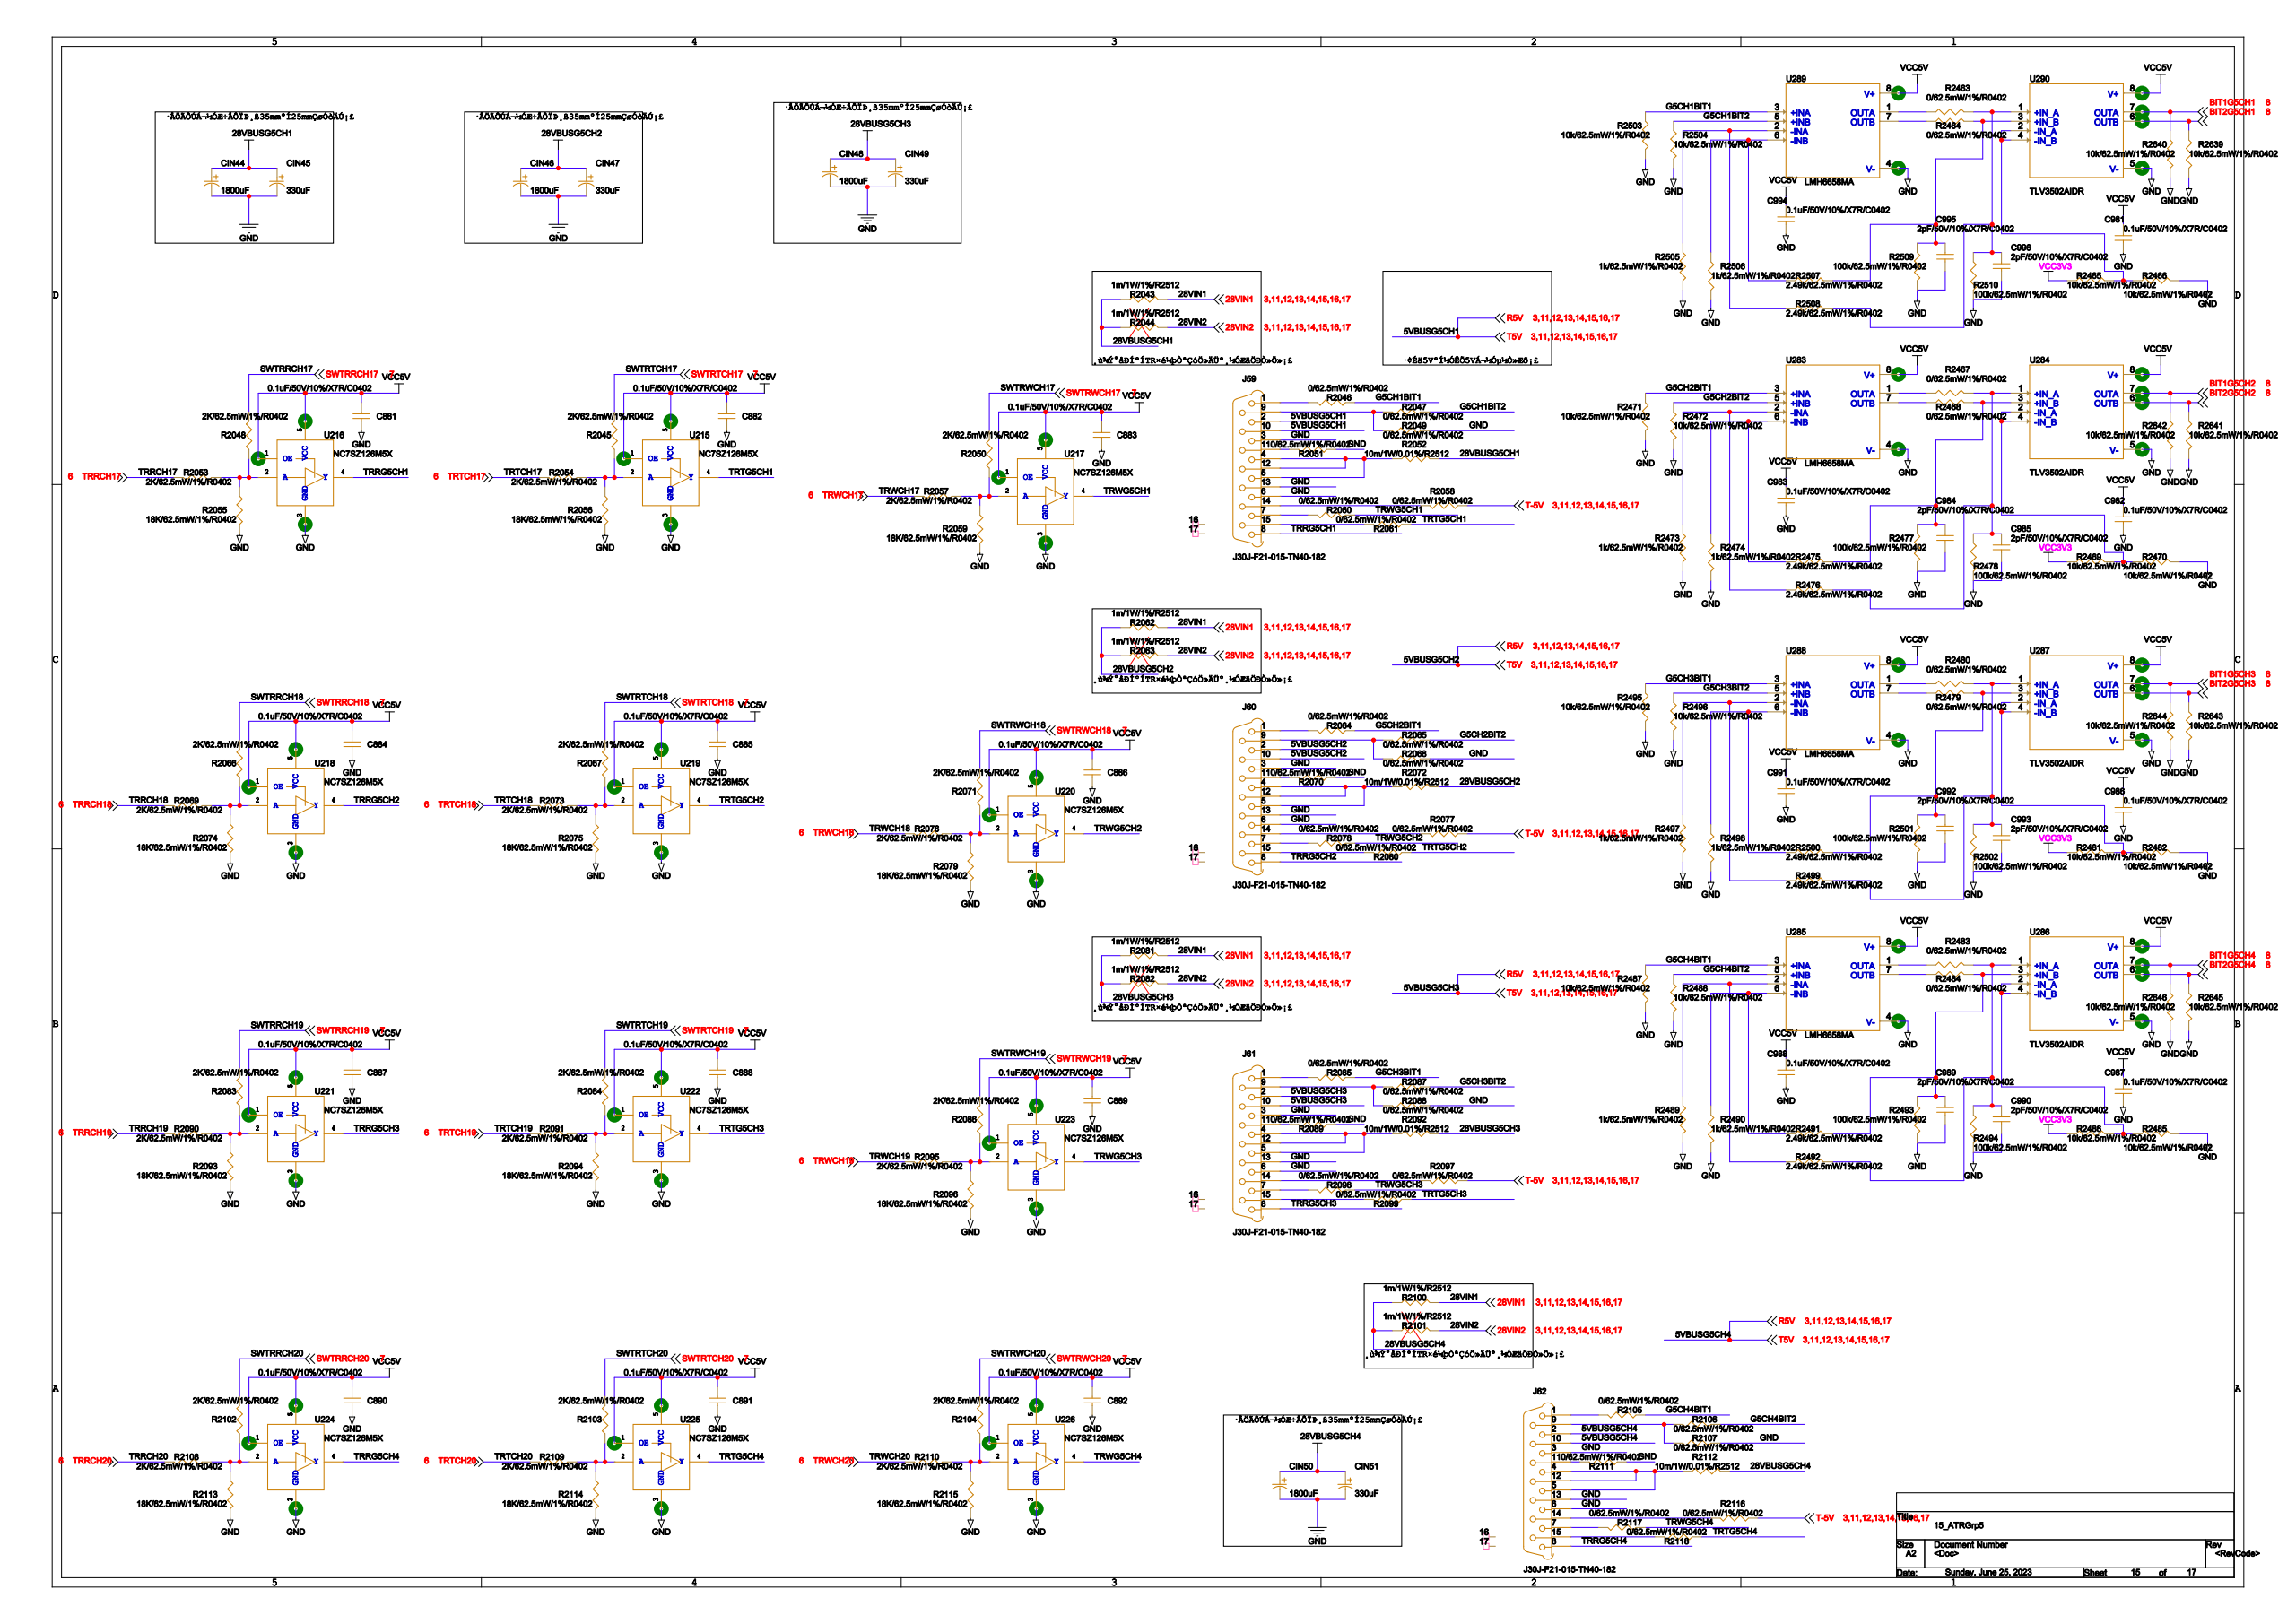Circuit board | Cadence Allegro | 1997 parts | 1536 nets | one sheet of the schematic
Parts on this sheet (reference | value | footprint):
C881 | 0.1uF/50V/10%/X7R/C0402 | 0402
C882 | 0.1uF/50V/10%/X7R/C0402 | 0402
C883 | 0.1uF/50V/10%/X7R/C0402 | 0402
C884 | 0.1uF/50V/10%/X7R/C0402 | 0402
C885 | 0.1uF/50V/10%/X7R/C0402 | 0402
C886 | 0.1uF/50V/10%/X7R/C0402 | 0402
C887 | 0.1uF/50V/10%/X7R/C0402 | 0402
C888 | 0.1uF/50V/10%/X7R/C0402 | 0402
C889 | 0.1uF/50V/10%/X7R/C0402 | 0402
C890 | 0.1uF/50V/10%/X7R/C0402 | 0402
C891 | 0.1uF/50V/10%/X7R/C0402 | 0402
C892 | 0.1uF/50V/10%/X7R/C0402 | 0402
C981 | 0.1uF/50V/10%/X7R/C0402 | 0402
C982 | 0.1uF/50V/10%/X7R/C0402 | 0402
C984 | 2pF/50V/10%/X7R/C0402 | 0402
C985 | 2pF/50V/10%/X7R/C0402 | 0402
C986 | 0.1uF/50V/10%/X7R/C0402 | 0402
C987 | 0.1uF/50V/10%/X7R/C0402 | 0402
C989 | 2pF/50V/10%/X7R/C0402 | 0402
C990 | 2pF/50V/10%/X7R/C0402 | 0402
C992 | 2pF/50V/10%/X7R/C0402 | 0402
C993 | 2pF/50V/10%/X7R/C0402 | 0402
C995 | 2pF/50V/10%/X7R/C0402 | 0402
C996 | 2pF/50V/10%/X7R/C0402 | 0402
CIN44 | ECF1HM182M27OTPO | AP-SMD_BD18-L27-W6_6-LS7_21
CIN45 | ECF1JM331G20OTPO | AP-SMD_BD10-L20-W6_6-LS7_21
CIN46 | ECF1HM182M27OTPO | AP-SMD_BD18-L27-W6_6-LS7_21
CIN47 | ECF1JM331G20OTPO | AP-SMD_BD10-L20-W6_6-LS7_21
CIN48 | ECF1HM182M27OTPO | AP-SMD_BD18-L27-W6_6-LS7_21
CIN49 | ECF1JM331G20OTPO | AP-SMD_BD10-L20-W6_6-LS7_21
CIN50 | ECF1HM182M27OTPO | AP-SMD_BD18-L27-W6_6-LS7_21
CIN51 | ECF1JM331G20OTPO | AP-SMD_BD10-L20-W6_6-LS7_21
J59 | J30J-F21-015-TN40-182 | J30J-F21-015-TN40-182
J60 | J30J-F21-015-TN40-182 | J30J-F21-015-TN40-182
J61 | J30J-F21-015-TN40-182 | J30J-F21-015-TN40-182
J62 | J30J-F21-015-TN40-182 | J30J-F21-015-TN40-182
R2043 | 1m/1W/1%/R2512 | 2512
R2044 | 1m/1W/1%/R2512 | 2512
R2045 | 2K/62.5mW/1%/R0402 | 0402
R2046 | 0/62.5mW/1%/R0402 | 0402
R2047 | 0/62.5mW/1%/R0402 | 0402
R2048 | 2K/62.5mW/1%/R0402 | 0402
R2049 | 0/62.5mW/1%/R0402 | 0402
R2050 | 2K/62.5mW/1%/R0402 | 0402
R2051 | 0/62.5mW/1%/R0402 | 0402
R2052 | 10m/1W/0.01%/R2512 | 2512
R2053 | 2K/62.5mW/1%/R0402 | 0402
R2054 | 2K/62.5mW/1%/R0402 | 0402
R2055 | 18K/62.5mW/1%/R0402 | 0402
R2056 | 18K/62.5mW/1%/R0402 | 0402
R2057 | 2K/62.5mW/1%/R0402 | 0402
R2058 | 0/62.5mW/1%/R0402 | 0402
R2059 | 18K/62.5mW/1%/R0402 | 0402
R2060 | 0/62.5mW/1%/R0402 | 0402
R2061 | 0/62.5mW/1%/R0402 | 0402
R2062 | 1m/1W/1%/R2512 | 2512
R2063 | 1m/1W/1%/R2512 | 2512
R2064 | 0/62.5mW/1%/R0402 | 0402
R2065 | 0/62.5mW/1%/R0402 | 0402
R2066 | 2K/62.5mW/1%/R0402 | 0402
R2067 | 2K/62.5mW/1%/R0402 | 0402
R2068 | 0/62.5mW/1%/R0402 | 0402
R2069 | 2K/62.5mW/1%/R0402 | 0402
R2070 | 0/62.5mW/1%/R0402 | 0402
R2071 | 2K/62.5mW/1%/R0402 | 0402
R2072 | 10m/1W/0.01%/R2512 | 2512
R2073 | 2K/62.5mW/1%/R0402 | 0402
R2074 | 18K/62.5mW/1%/R0402 | 0402
R2075 | 18K/62.5mW/1%/R0402 | 0402
R2076 | 2K/62.5mW/1%/R0402 | 0402
R2077 | 0/62.5mW/1%/R0402 | 0402
R2078 | 0/62.5mW/1%/R0402 | 0402
R2079 | 18K/62.5mW/1%/R0402 | 0402
R2080 | 0/62.5mW/1%/R0402 | 0402
R2081 | 1m/1W/1%/R2512 | 2512
R2082 | 1m/1W/1%/R2512 | 2512
R2083 | 2K/62.5mW/1%/R0402 | 0402
R2084 | 2K/62.5mW/1%/R0402 | 0402
R2085 | 0/62.5mW/1%/R0402 | 0402
R2086 | 2K/62.5mW/1%/R0402 | 0402
R2087 | 0/62.5mW/1%/R0402 | 0402
R2088 | 0/62.5mW/1%/R0402 | 0402
R2089 | 0/62.5mW/1%/R0402 | 0402
R2090 | 2K/62.5mW/1%/R0402 | 0402
R2091 | 2K/62.5mW/1%/R0402 | 0402
R2092 | 10m/1W/0.01%/R2512 | 2512
R2093 | 18K/62.5mW/1%/R0402 | 0402
R2094 | 18K/62.5mW/1%/R0402 | 0402
R2095 | 2K/62.5mW/1%/R0402 | 0402
R2096 | 18K/62.5mW/1%/R0402 | 0402
R2097 | 0/62.5mW/1%/R0402 | 0402
R2098 | 0/62.5mW/1%/R0402 | 0402
R2099 | 0/62.5mW/1%/R0402 | 0402
R2100 | 1m/1W/1%/R2512 | 2512
R2101 | 1m/1W/1%/R2512 | 2512
R2102 | 2K/62.5mW/1%/R0402 | 0402
R2103 | 2K/62.5mW/1%/R0402 | 0402
R2104 | 2K/62.5mW/1%/R0402 | 0402
R2105 | 0/62.5mW/1%/R0402 | 0402
R2106 | 0/62.5mW/1%/R0402 | 0402
R2107 | 0/62.5mW/1%/R0402 | 0402
R2108 | 2K/62.5mW/1%/R0402 | 0402
R2109 | 2K/62.5mW/1%/R0402 | 0402
R2110 | 2K/62.5mW/1%/R0402 | 0402
R2111 | 0/62.5mW/1%/R0402 | 0402
R2112 | 10m/1W/0.01%/R2512 | 2512
R2113 | 18K/62.5mW/1%/R0402 | 0402
R2114 | 18K/62.5mW/1%/R0402 | 0402
R2115 | 18K/62.5mW/1%/R0402 | 0402
R2116 | 0/62.5mW/1%/R0402 | 0402
R2117 | 0/62.5mW/1%/R0402 | 0402
R2118 | 0/62.5mW/1%/R0402 | 0402
R2463 | 0/62.5mW/1%/R0402 | 0402
R2464 | 0/62.5mW/1%/R0402 | 0402
R2465 | 10k/62.5mW/1%/R0402 | 0402
R2466 | 10k/62.5mW/1%/R0402 | 0402
R2467 | 0/62.5mW/1%/R0402 | 0402
R2468 | 0/62.5mW/1%/R0402 | 0402
R2469 | 10k/62.5mW/1%/R0402 | 0402
R2470 | 10k/62.5mW/1%/R0402 | 0402
R2471 | 10k/62.5mW/1%/R0402 | 0402
R2472 | 10k/62.5mW/1%/R0402 | 0402
R2473 | 1K/62.5mW/1%/R0402 | 0402
R2474 | 1K/62.5mW/1%/R0402 | 0402
R2476 | 2.49k/62.5mW/1%/R0402 | 0402
R2477 | 100k/62.5mW/1%/R0402 | 0402
R2478 | 100k/62.5mW/1%/R0402 | 0402
R2479 | 0/62.5mW/1%/R0402 | 0402
R2480 | 0/62.5mW/1%/R0402 | 0402
R2481 | 10k/62.5mW/1%/R0402 | 0402
R2482 | 10k/62.5mW/1%/R0402 | 0402
R2483 | 0/62.5mW/1%/R0402 | 0402
R2484 | 0/62.5mW/1%/R0402 | 0402
R2485 | 10k/62.5mW/1%/R0402 | 0402
R2486 | 10k/62.5mW/1%/R0402 | 0402
R2487 | 10k/62.5mW/1%/R0402 | 0402
R2488 | 10k/62.5mW/1%/R0402 | 0402
R2489 | 1K/62.5mW/1%/R0402 | 0402
R2490 | 1K/62.5mW/1%/R0402 | 0402
R2492 | 2.49k/62.5mW/1%/R0402 | 0402
R2493 | 100k/62.5mW/1%/R0402 | 0402
R2494 | 100k/62.5mW/1%/R0402 | 0402
R2495 | 10k/62.5mW/1%/R0402 | 0402
R2496 | 10k/62.5mW/1%/R0402 | 0402
R2497 | 1K/62.5mW/1%/R0402 | 0402
R2498 | 1K/62.5mW/1%/R0402 | 0402
R2499 | 2.49k/62.5mW/1%/R0402 | 0402
R2500 | 2.49k/62.5mW/1%/R0402 | 0402
R2501 | 100k/62.5mW/1%/R0402 | 0402
R2502 | 100k/62.5mW/1%/R0402 | 0402
R2503 | 10k/62.5mW/1%/R0402 | 0402
R2504 | 10k/62.5mW/1%/R0402 | 0402
R2505 | 1K/62.5mW/1%/R0402 | 0402
R2506 | 1K/62.5mW/1%/R0402 | 0402
R2508 | 2.49k/62.5mW/1%/R0402 | 0402
R2509 | 100k/62.5mW/1%/R0402 | 0402
R2510 | 100k/62.5mW/1%/R0402 | 0402
R2639 | 10k/62.5mW/1%/R0402 | 0402
R2640 | 10k/62.5mW/1%/R0402 | 0402
R2641 | 10k/62.5mW/1%/R0402 | 0402
R2642 | 10k/62.5mW/1%/R0402 | 0402
R2643 | 10k/62.5mW/1%/R0402 | 0402
R2644 | 10k/62.5mW/1%/R0402 | 0402
R2645 | 10k/62.5mW/1%/R0402 | 0402
R2646 | 10k/62.5mW/1%/R0402 | 0402
U215 | NC7SZ126M5X | SOT-23-5
U216 | NC7SZ126M5X | SOT-23-5
U217 | NC7SZ126M5X | SOT-23-5
U218 | NC7SZ126M5X | SOT-23-5
U219 | NC7SZ126M5X | SOT-23-5
U220 | NC7SZ126M5X | SOT-23-5
U221 | NC7SZ126M5X | SOT-23-5
U222 | NC7SZ126M5X | SOT-23-5
U223 | NC7SZ126M5X | SOT-23-5
U224 | NC7SZ126M5X | SOT-23-5
U225 | NC7SZ126M5X | SOT-23-5
U226 | NC7SZ126M5X | SOT-23-5
U283 | LMH6658MA | SOIC127P599X175-8N
U285 | LMH6658MA | SOIC127P599X175-8N
U287 | TLV3502AIDR | SOIC127P599X175-8N
U289 | LMH6658MA | SOIC127P599X175-8N
Nets of these parts (net: part-pin ...):
3.3V: R2465-1 R2469-1 R2481-1 R2486-1
AGND: C881-2 C882-2 C883-2 C884-2 C885-2 C886-2 C887-2 C888-2 C889-2 C890-2 C891-2 C892-2 C981-2 C982-2 C984-2 C985-2 C986-2 C987-2 C989-2 C990-2 C992-2 C993-2 C995-2 C996-2 CIN44-2 CIN45-2 CIN46-2 CIN47-2 CIN48-2 CIN49-2 CIN50-2 CIN51-2 J59-3 J59-6 J59-13 J60-3 J60-6 J60-13 J61-3 J61-6 J61-13 J62-3 J62-6 J62-13 R2049-1 R2051-1 R2055-1 R2056-1 R2059-1 R2068-1 R2070-1 R2074-1 R2075-1 R2079-1 R2088-1 R2089-1 R2093-1 R2094-1 R2096-1 R2107-1 R2111-1 R2113-1 R2114-1 R2115-1 R2466-2 R2470-2 R2471-2 R2472-2 R2473-2 R2474-2 R2477-2 R2478-2 R2482-2 R2485-2 R2487-2 R2488-2 R2489-2 R2490-2 R2493-2 R2494-2 R2495-2 R2496-2 R2497-2 R2498-2 R2501-2 R2502-2 R2503-2 R2504-2 R2505-2 R2506-2 R2509-2 R2510-2 R2639-2 R2640-2 R2641-2 R2642-2 R2643-2 R2644-2 R2645-2 R2646-2 U215-3 U216-3 U217-3 U218-3 U219-3 U220-3 U221-3 U222-3 U223-3 U224-3 U225-3 U226-3 U283-4 U285-4 U287-5 U289-4
VCC5V: C881-1 C882-1 C883-1 C884-1 C885-1 C886-1 C887-1 C888-1 C889-1 C890-1 C891-1 C892-1 C981-1 C982-1 C986-1 C987-1 U215-1 U215-5 U216-1 U216-5 U217-1 U217-5 U218-1 U218-5 U219-1 U219-5 U220-1 U220-5 U221-1 U221-5 U222-1 U222-5 U223-1 U223-5 U224-1 U224-5 U225-1 U225-5 U226-1 U226-5 U283-8 U285-8 U287-8 U289-8
N24406183: R2474-1 U283-6
N24406193: C984-1 R2468-2 R2477-1
N24406171: R2473-1 R2476-1 U283-2
N24406191: C985-1 R2467-2 R2476-2 R2478-1
N24406737: R2490-1 U285-6
N24406747: C989-1 R2484-2 R2493-1
N24406725: R2489-1 R2492-1 U285-2
N24406745: C990-1 R2483-2 R2492-2 R2494-1
N24406549: R2497-1 R2499-1
N24406565: C993-1 R2480-2 R2499-2 R2502-1 U287-1
N24406553: R2498-1 R2500-1
N24406567: C992-1 R2479-2 R2500-2 R2501-1 U287-3
N24406003: R2506-1 U289-6
N24406013: C995-1 R2464-2 R2509-1
N24405999: R2505-1 R2508-1 U289-2
N24406011: C996-1 R2463-2 R2508-2 R2510-1
G5CH2BIT1: R2064-1 R2471-1 U283-3
G5CH2BIT2: R2065-1 R2472-1 U283-5
N24406187: R2467-1 U283-1
N24406189: R2468-1 U283-7
G5CH4BIT1: R2105-1 R2487-1 U285-3
G5CH4BIT2: R2106-1 R2488-1 U285-5
N24406741: R2483-1 U285-1
N24406743: R2484-1 U285-7
G5CH3BIT1: R2085-1 R2495-1
G5CH3BIT2: R2087-1 R2496-1
N24406561: R2480-1
N24406563: R2479-1
G5CH1BIT1: R2046-1 R2503-1 U289-3
G5CH1BIT2: R2047-1 R2504-1 U289-5
N24406007: R2463-1 U289-1
N24406009: R2464-1 U289-7
N24406245: R2469-2 R2470-1
BIT1G5CH2: R2642-1
BIT2G5CH2: R2641-1
N24406799: R2485-1 R2486-2
BIT1G5CH4: R2646-1
BIT2G5CH4: R2645-1
N24406619: R2481-2 R2482-1 U287-2 U287-4
BIT1G5CH3: R2644-1 U287-7
BIT2G5CH3: R2643-1 U287-6
N24406065: R2465-2 R2466-1
BIT1G5CH1: R2640-1
BIT2G5CH1: R2639-1
R5V: J59-2 J59-10 J60-2 J60-10 J61-2 J61-10 J62-2 J62-10
N23730929: J59-1 R2046-2
N23730942: J59-11 R2051-2
N23730944: J59-4 J59-5 J59-12 R2052-1
N23730956: J59-14 R2058-2
N23730960: J59-15 R2061-2
N23730958: J59-7 R2060-2
TRRG5CH1: J59-8 U216-4
N23730931: J59-9 R2047-2 R2049-2
N23731488: J60-1 R2064-2
N23731501: J60-11 R2070-2
N23731503: J60-4 J60-5 J60-12 R2072-1
N23731515: J60-14 R2077-2
N23731519: J60-15 R2080-2
N23731517: J60-7 R2078-2
TRRG5CH2: J60-8 U218-4
N23731490: J60-9 R2065-2 R2068-2
N23732115: J61-1 R2085-2
N23732128: J61-11 R2089-2
N23732130: J61-4 J61-5 J61-12 R2092-1
N23732142: J61-14 R2097-2
N23732146: J61-15 R2099-2
N23732144: J61-7 R2098-2
TRRG5CH3: J61-8 U221-4
N23732117: J61-9 R2087-2 R2088-2
N23732747: J62-1 R2105-2
N23732760: J62-11 R2111-2
N23732762: J62-4 J62-5 J62-12 R2112-1
N23732774: J62-14 R2116-2
N23732778: J62-15 R2118-2
N23732776: J62-7 R2117-2
TRRG5CH4: J62-8 U224-4
N23732749: J62-9 R2106-2 R2107-2
28VIN1: R2043-2 R2062-2 R2081-2 R2100-2
T-5V: R2058-1 R2077-1 R2097-1 R2116-1
28VIN2: R2044-2 R2063-2 R2082-2 R2101-2
28VBUSG5CH1: CIN44-1 CIN45-1 R2043-1 R2044-1 R2052-2
28VBUSG5CH2: CIN46-1 CIN47-1 R2062-1 R2063-1 R2072-2
28VBUSG5CH3: CIN48-1 CIN49-1 R2081-1 R2082-1 R2092-2
28VBUSG5CH4: CIN50-1 CIN51-1 R2100-1 R2101-1 R2112-2
SWTRTCH17: R2045-1
N24013764: R2045-2 R2054-2 R2056-2 U215-2
SWTRRCH17: R2048-1
N24014744: R2048-2 R2053-2 R2055-2 U216-2
SWTRWCH17: R2050-1
N24014252: R2050-2 R2057-2 R2059-2 U217-2
TRRCH17: R2053-1
TRTCH17: R2054-1
TRWCH17: R2057-1
SWTRRCH18: R2066-1
N24014862: R2066-2 R2069-2 R2074-2 U218-2
SWTRTCH18: R2067-1
N24013882: R2067-2 R2073-2 R2075-2 U219-2
TRRCH18: R2069-1
SWTRWCH18: R2071-1
N24014374: R2071-2 R2076-2 R2079-2 U220-2
TRTCH18: R2073-1
TRWCH18: R2076-1
SWTRRCH19: R2083-1
N24014988: R2083-2 R2090-2 R2093-2 U221-2
SWTRTCH19: R2084-1
N24014008: R2084-2 R2091-2 R2094-2 U222-2
SWTRWCH19: R2086-1
N24014496: R2086-2 R2095-2 R2096-2 U223-2
TRRCH19: R2090-1
TRTCH19: R2091-1
TRWCH19: R2095-1
SWTRRCH20: R2102-1
N24015106: R2102-2 R2108-2 R2113-2 U224-2
SWTRTCH20: R2103-1
N24014130: R2103-2 R2109-2 R2114-2 U225-2
SWTRWCH20: R2104-1
N24014618: R2104-2 R2110-2 R2115-2 U226-2
TRRCH20: R2108-1
TRTCH20: R2109-1
TRWCH20: R2110-1
TRTG5CH1: R2061-1 U215-4
TRWG5CH1: R2060-1 U217-4
TRTG5CH2: R2080-1 U219-4
TRWG5CH2: R2078-1 U220-4
TRTG5CH3: R2099-1 U222-4
TRWG5CH3: R2098-1 U223-4
TRTG5CH4: R2118-1 U225-4
TRWG5CH4: R2117-1 U226-4